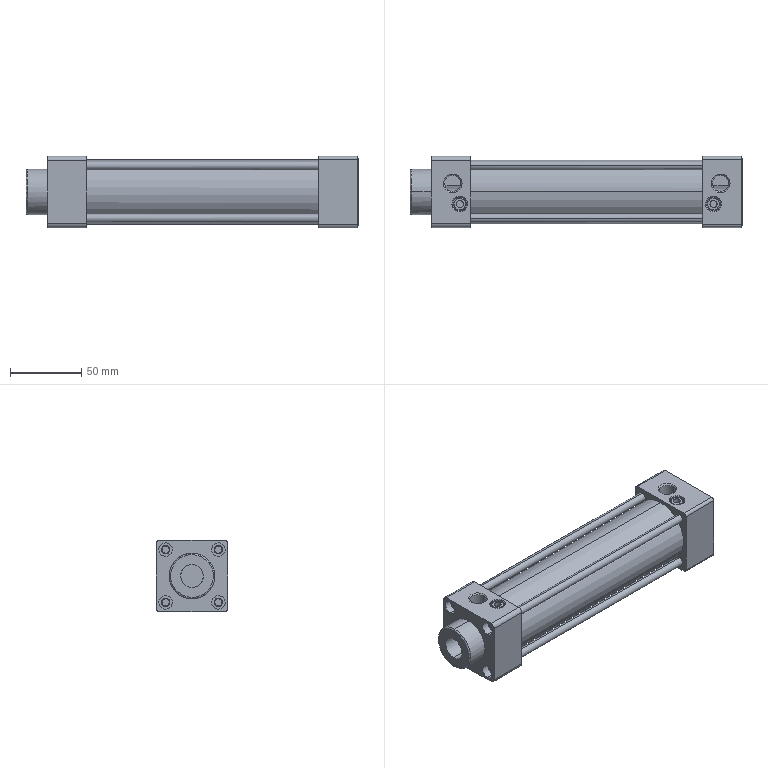Part | SolidWorks | features BaseBody 1 | 1 solid | 147 faces | box 233 x 50 x 50 mm | volume 209735 mm3 | cylinder 76 | plane 41 | cone 28 | torus 2 | commonest cylinder face diameters 4.917 x16 9.5 x16 6 x12 4 x4 5 x4 9.1 x4